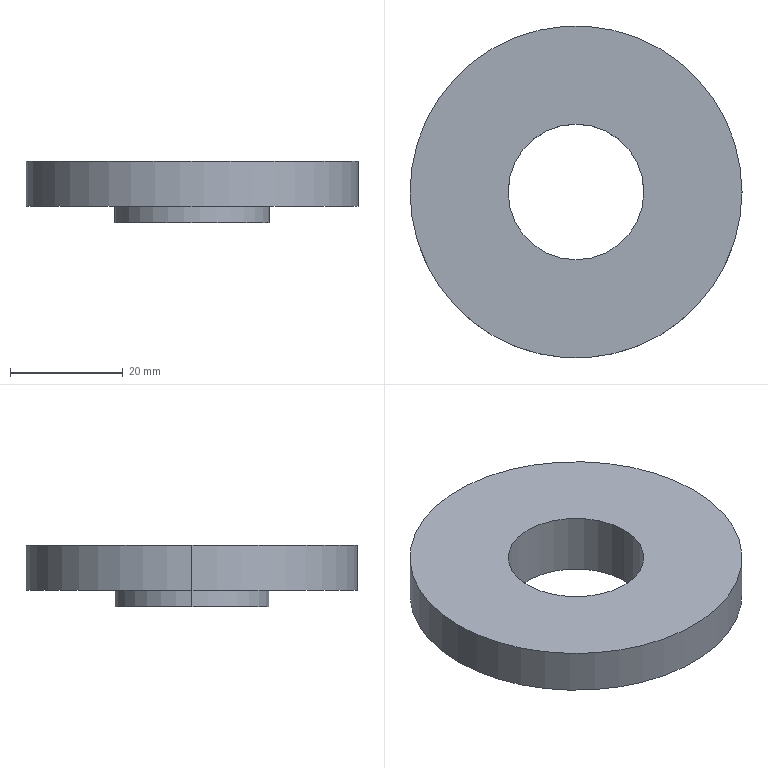Part | STEP file | LM-05-1133_default | 1 solid | 9 faces | box 59 x 59 x 11 mm | volume 18636 mm3 | cylinder 6 | plane 3 | commonest cylinder face diameters 24.1 x2 27.5 x2 59 x2
STEP:
#1=CARTESIAN_POINT('',(0.,0.,0.));
#2=DIRECTION('',(0.,0.,1.));
#3=DIRECTION('',(1.,0.,0.));
#4=AXIS2_PLACEMENT_3D('',#1,#2,#3);
#5=CARTESIAN_POINT('',(-13.75,0.,-2.));
#6=VERTEX_POINT('',#5);
#7=CARTESIAN_POINT('',(13.75,0.,-2.));
#8=VERTEX_POINT('',#7);
#9=CARTESIAN_POINT('',(0.,0.,-2.));
#10=DIRECTION('',(0.,0.,-1.));
#11=DIRECTION('',(-1.,0.,0.));
#12=AXIS2_PLACEMENT_3D('',#9,#10,#11);
#13=CIRCLE('',#12,13.75);
#14=CARTESIAN_POINT('',(0.,0.,6.));
#15=DIRECTION('',(0.,0.,-1.));
#16=DIRECTION('',(-1.,0.,0.));
#17=AXIS2_PLACEMENT_3D('',#14,#15,#16);
#18=CYLINDRICAL_SURFACE('',#17,13.75);
#19=CARTESIAN_POINT('',(0.,8.));
#20=DIRECTION('',(1.,0.));
#21=VECTOR('',#20,1.);
#22=LINE('',#19,#21);
#23=(GEOMETRIC_REPRESENTATION_CONTEXT(2)PARAMETRIC_REPRESENTATION_CONTEXT()REPRESENTATION_CONTEXT('',''));
#24=DEFINITIONAL_REPRESENTATION('',(#22),#23);
#25=PCURVE('',#18,#24);
#26=CARTESIAN_POINT('',(13.75,0.,-2.));
#27=DIRECTION('',(0.,0.,-1.));
#28=DIRECTION('',(-1.,0.,0.));
#29=AXIS2_PLACEMENT_3D('',#26,#27,#28);
#30=PLANE('',#29);
#31=CARTESIAN_POINT('',(13.75,0.));
#32=DIRECTION('',(1.,0.));
#33=AXIS2_PLACEMENT_2D('',#31,#32);
#34=CIRCLE('',#33,13.75);
#35=(GEOMETRIC_REPRESENTATION_CONTEXT(2)PARAMETRIC_REPRESENTATION_CONTEXT()REPRESENTATION_CONTEXT('',''));
#36=DEFINITIONAL_REPRESENTATION('',(#34),#35);
#37=PCURVE('',#30,#36);
#38=SURFACE_CURVE('',#13,(#25,#37),.PCURVE_S1.);
#39=EDGE_CURVE('',#6,#8,#38,.T.);
#40=ORIENTED_EDGE('',*,*,#39,.T.);
#41=CARTESIAN_POINT('',(13.75,0.,-5.));
#42=VERTEX_POINT('',#41);
#43=CARTESIAN_POINT('',(13.75,0.,6.));
#44=DIRECTION('',(0.,0.,-1.));
#45=VECTOR('',#44,1.);
#46=LINE('',#43,#45);
#47=CARTESIAN_POINT('',(3.142,0.));
#48=DIRECTION('',(0.,1.));
#49=VECTOR('',#48,1.);
#50=LINE('',#47,#49);
#51=(GEOMETRIC_REPRESENTATION_CONTEXT(2)PARAMETRIC_REPRESENTATION_CONTEXT()REPRESENTATION_CONTEXT('',''));
#52=DEFINITIONAL_REPRESENTATION('',(#50),#51);
#53=PCURVE('',#18,#52);
#54=CARTESIAN_POINT('',(0.,0.,6.));
#55=DIRECTION('',(0.,0.,-1.));
#56=DIRECTION('',(-1.,0.,0.));
#57=AXIS2_PLACEMENT_3D('',#54,#55,#56);
#58=CYLINDRICAL_SURFACE('',#57,13.75);
#59=CARTESIAN_POINT('',(3.142,0.));
#60=DIRECTION('',(0.,1.));
#61=VECTOR('',#60,1.);
#62=LINE('',#59,#61);
#63=(GEOMETRIC_REPRESENTATION_CONTEXT(2)PARAMETRIC_REPRESENTATION_CONTEXT()REPRESENTATION_CONTEXT('',''));
#64=DEFINITIONAL_REPRESENTATION('',(#62),#63);
#65=PCURVE('',#58,#64);
#66=SURFACE_CURVE('',#46,(#53,#65),.PCURVE_S1.);
#67=EDGE_CURVE('',#8,#42,#66,.T.);
#68=ORIENTED_EDGE('',*,*,#67,.T.);
#69=CARTESIAN_POINT('',(-13.75,0.,-5.));
#70=VERTEX_POINT('',#69);
#71=CARTESIAN_POINT('',(0.,0.,-5.));
#72=DIRECTION('',(0.,0.,-1.));
#73=DIRECTION('',(-1.,0.,0.));
#74=AXIS2_PLACEMENT_3D('',#71,#72,#73);
#75=CIRCLE('',#74,13.75);
#76=CARTESIAN_POINT('',(0.,11.));
#77=DIRECTION('',(1.,0.));
#78=VECTOR('',#77,1.);
#79=LINE('',#76,#78);
#80=(GEOMETRIC_REPRESENTATION_CONTEXT(2)PARAMETRIC_REPRESENTATION_CONTEXT()REPRESENTATION_CONTEXT('',''));
#81=DEFINITIONAL_REPRESENTATION('',(#79),#80);
#82=PCURVE('',#18,#81);
#83=CARTESIAN_POINT('',(12.05,0.,-5.));
#84=DIRECTION('',(0.,0.,-1.));
#85=DIRECTION('',(-1.,0.,0.));
#86=AXIS2_PLACEMENT_3D('',#83,#84,#85);
#87=PLANE('',#86);
#88=CARTESIAN_POINT('',(12.05,0.));
#89=DIRECTION('',(1.,0.));
#90=AXIS2_PLACEMENT_2D('',#88,#89);
#91=CIRCLE('',#90,13.75);
#92=(GEOMETRIC_REPRESENTATION_CONTEXT(2)PARAMETRIC_REPRESENTATION_CONTEXT()REPRESENTATION_CONTEXT('',''));
#93=DEFINITIONAL_REPRESENTATION('',(#91),#92);
#94=PCURVE('',#87,#93);
#95=SURFACE_CURVE('',#75,(#82,#94),.PCURVE_S1.);
#96=EDGE_CURVE('',#70,#42,#95,.T.);
#97=ORIENTED_EDGE('',*,*,#96,.F.);
#98=CARTESIAN_POINT('',(-13.75,0.,6.));
#99=DIRECTION('',(0.,0.,-1.));
#100=VECTOR('',#99,1.);
#101=LINE('',#98,#100);
#102=CARTESIAN_POINT('',(0.,0.));
#103=DIRECTION('',(0.,1.));
#104=VECTOR('',#103,1.);
#105=LINE('',#102,#104);
#106=(GEOMETRIC_REPRESENTATION_CONTEXT(2)PARAMETRIC_REPRESENTATION_CONTEXT()REPRESENTATION_CONTEXT('',''));
#107=DEFINITIONAL_REPRESENTATION('',(#105),#106);
#108=PCURVE('',#18,#107);
#109=CARTESIAN_POINT('',(6.283,0.));
#110=DIRECTION('',(0.,1.));
#111=VECTOR('',#110,1.);
#112=LINE('',#109,#111);
#113=(GEOMETRIC_REPRESENTATION_CONTEXT(2)PARAMETRIC_REPRESENTATION_CONTEXT()REPRESENTATION_CONTEXT('',''));
#114=DEFINITIONAL_REPRESENTATION('',(#112),#113);
#115=PCURVE('',#58,#114);
#116=SURFACE_CURVE('',#101,(#108,#115),.PCURVE_S1.);
#117=EDGE_CURVE('',#6,#70,#116,.T.);
#118=ORIENTED_EDGE('',*,*,#117,.F.);
#119=EDGE_LOOP('',(#40,#68,#97,#118));
#120=FACE_BOUND('',#119,.T.);
#121=ADVANCED_FACE('',(#120),#18,.T.);
#122=CARTESIAN_POINT('',(-12.05,0.,6.));
#123=VERTEX_POINT('',#122);
#124=CARTESIAN_POINT('',(-12.05,0.,-5.));
#125=VERTEX_POINT('',#124);
#126=CARTESIAN_POINT('',(-12.05,0.,6.));
#127=DIRECTION('',(0.,0.,-1.));
#128=VECTOR('',#127,1.);
#129=LINE('',#126,#128);
#130=CARTESIAN_POINT('',(0.,0.,6.));
#131=DIRECTION('',(0.,0.,-1.));
#132=DIRECTION('',(-1.,0.,0.));
#133=AXIS2_PLACEMENT_3D('',#130,#131,#132);
#134=CYLINDRICAL_SURFACE('',#133,12.05);
#135=CARTESIAN_POINT('',(6.283,0.));
#136=DIRECTION('',(0.,1.));
#137=VECTOR('',#136,1.);
#138=LINE('',#135,#137);
#139=(GEOMETRIC_REPRESENTATION_CONTEXT(2)PARAMETRIC_REPRESENTATION_CONTEXT()REPRESENTATION_CONTEXT('',''));
#140=DEFINITIONAL_REPRESENTATION('',(#138),#139);
#141=PCURVE('',#134,#140);
#142=CARTESIAN_POINT('',(0.,0.,6.));
#143=DIRECTION('',(0.,0.,-1.));
#144=DIRECTION('',(-1.,0.,0.));
#145=AXIS2_PLACEMENT_3D('',#142,#143,#144);
#146=CYLINDRICAL_SURFACE('',#145,12.05);
#147=CARTESIAN_POINT('',(0.,0.));
#148=DIRECTION('',(0.,1.));
#149=VECTOR('',#148,1.);
#150=LINE('',#147,#149);
#151=(GEOMETRIC_REPRESENTATION_CONTEXT(2)PARAMETRIC_REPRESENTATION_CONTEXT()REPRESENTATION_CONTEXT('',''));
#152=DEFINITIONAL_REPRESENTATION('',(#150),#151);
#153=PCURVE('',#146,#152);
#154=SURFACE_CURVE('',#129,(#141,#153),.PCURVE_S1.);
#155=EDGE_CURVE('',#123,#125,#154,.T.);
#156=ORIENTED_EDGE('',*,*,#155,.T.);
#157=CARTESIAN_POINT('',(12.05,0.,-5.));
#158=VERTEX_POINT('',#157);
#159=CARTESIAN_POINT('',(0.,0.,-5.));
#160=DIRECTION('',(0.,0.,-1.));
#161=DIRECTION('',(-1.,0.,0.));
#162=AXIS2_PLACEMENT_3D('',#159,#160,#161);
#163=CIRCLE('',#162,12.05);
#164=CARTESIAN_POINT('',(0.,11.));
#165=DIRECTION('',(1.,0.));
#166=VECTOR('',#165,1.);
#167=LINE('',#164,#166);
#168=(GEOMETRIC_REPRESENTATION_CONTEXT(2)PARAMETRIC_REPRESENTATION_CONTEXT()REPRESENTATION_CONTEXT('',''));
#169=DEFINITIONAL_REPRESENTATION('',(#167),#168);
#170=PCURVE('',#134,#169);
#171=CARTESIAN_POINT('',(12.05,0.));
#172=DIRECTION('',(1.,0.));
#173=AXIS2_PLACEMENT_2D('',#171,#172);
#174=CIRCLE('',#173,12.05);
#175=(GEOMETRIC_REPRESENTATION_CONTEXT(2)PARAMETRIC_REPRESENTATION_CONTEXT()REPRESENTATION_CONTEXT('',''));
#176=DEFINITIONAL_REPRESENTATION('',(#174),#175);
#177=PCURVE('',#87,#176);
#178=SURFACE_CURVE('',#163,(#170,#177),.PCURVE_S1.);
#179=EDGE_CURVE('',#158,#125,#178,.T.);
#180=ORIENTED_EDGE('',*,*,#179,.F.);
#181=CARTESIAN_POINT('',(12.05,0.,6.));
#182=VERTEX_POINT('',#181);
#183=CARTESIAN_POINT('',(12.05,0.,6.));
#184=DIRECTION('',(0.,0.,-1.));
#185=VECTOR('',#184,1.);
#186=LINE('',#183,#185);
#187=CARTESIAN_POINT('',(3.142,0.));
#188=DIRECTION('',(0.,1.));
#189=VECTOR('',#188,1.);
#190=LINE('',#187,#189);
#191=(GEOMETRIC_REPRESENTATION_CONTEXT(2)PARAMETRIC_REPRESENTATION_CONTEXT()REPRESENTATION_CONTEXT('',''));
#192=DEFINITIONAL_REPRESENTATION('',(#190),#191);
#193=PCURVE('',#134,#192);
#194=CARTESIAN_POINT('',(3.142,0.));
#195=DIRECTION('',(0.,1.));
#196=VECTOR('',#195,1.);
#197=LINE('',#194,#196);
#198=(GEOMETRIC_REPRESENTATION_CONTEXT(2)PARAMETRIC_REPRESENTATION_CONTEXT()REPRESENTATION_CONTEXT('',''));
#199=DEFINITIONAL_REPRESENTATION('',(#197),#198);
#200=PCURVE('',#146,#199);
#201=SURFACE_CURVE('',#186,(#193,#200),.PCURVE_S1.);
#202=EDGE_CURVE('',#182,#158,#201,.T.);
#203=ORIENTED_EDGE('',*,*,#202,.F.);
#204=CARTESIAN_POINT('',(0.,0.,6.));
#205=DIRECTION('',(0.,0.,-1.));
#206=DIRECTION('',(-1.,0.,0.));
#207=AXIS2_PLACEMENT_3D('',#204,#205,#206);
#208=CIRCLE('',#207,12.05);
#209=CARTESIAN_POINT('',(0.,0.));
#210=DIRECTION('',(1.,0.));
#211=VECTOR('',#210,1.);
#212=LINE('',#209,#211);
#213=(GEOMETRIC_REPRESENTATION_CONTEXT(2)PARAMETRIC_REPRESENTATION_CONTEXT()REPRESENTATION_CONTEXT('',''));
#214=DEFINITIONAL_REPRESENTATION('',(#212),#213);
#215=PCURVE('',#134,#214);
#216=CARTESIAN_POINT('',(29.5,0.,6.));
#217=DIRECTION('',(0.,0.,1.));
#218=DIRECTION('',(1.,0.,0.));
#219=AXIS2_PLACEMENT_3D('',#216,#217,#218);
#220=PLANE('',#219);
#221=CARTESIAN_POINT('',(-41.55,0.));
#222=CARTESIAN_POINT('',(-41.55,20.871));
#223=CARTESIAN_POINT('',(-23.475,10.436));
#224=CARTESIAN_POINT('',(-5.4,0.));
#225=CARTESIAN_POINT('',(-23.475,-10.436));
#226=CARTESIAN_POINT('',(-41.55,-20.871));
#227=CARTESIAN_POINT('',(-41.55,0.));
#228=(BOUNDED_CURVE()B_SPLINE_CURVE(2,(#221,#222,#223,#224,#225,#226,#227),.UNSPECIFIED.,.T.,.F.)B_SPLINE_CURVE_WITH_KNOTS((1,2,2,2,2,1),(-2.094,0.,2.094,4.189,6.283,8.378),.UNSPECIFIED.)CURVE()GEOMETRIC_REPRESENTATION_ITEM()RATIONAL_B_SPLINE_CURVE((1.,0.5,1.,0.5,1.,0.5,1.))REPRESENTATION_ITEM(''));
#229=(GEOMETRIC_REPRESENTATION_CONTEXT(2)PARAMETRIC_REPRESENTATION_CONTEXT()REPRESENTATION_CONTEXT('',''));
#230=DEFINITIONAL_REPRESENTATION('',(#228),#229);
#231=PCURVE('',#220,#230);
#232=SURFACE_CURVE('',#208,(#215,#231),.PCURVE_S1.);
#233=EDGE_CURVE('',#182,#123,#232,.T.);
#234=ORIENTED_EDGE('',*,*,#233,.T.);
#235=EDGE_LOOP('',(#156,#180,#203,#234));
#236=FACE_BOUND('',#235,.F.);
#237=ADVANCED_FACE('',(#236),#134,.F.);
#238=CARTESIAN_POINT('',(-29.5,0.,6.));
#239=VERTEX_POINT('',#238);
#240=CARTESIAN_POINT('',(29.5,0.,6.));
#241=VERTEX_POINT('',#240);
#242=CARTESIAN_POINT('',(0.,0.,6.));
#243=DIRECTION('',(0.,0.,-1.));
#244=DIRECTION('',(-1.,0.,0.));
#245=AXIS2_PLACEMENT_3D('',#242,#243,#244);
#246=CIRCLE('',#245,29.5);
#247=CARTESIAN_POINT('',(0.,0.,6.));
#248=DIRECTION('',(0.,0.,-1.));
#249=DIRECTION('',(-1.,0.,0.));
#250=AXIS2_PLACEMENT_3D('',#247,#248,#249);
#251=CYLINDRICAL_SURFACE('',#250,29.5);
#252=CARTESIAN_POINT('',(0.,0.));
#253=DIRECTION('',(1.,0.));
#254=VECTOR('',#253,1.);
#255=LINE('',#252,#254);
#256=(GEOMETRIC_REPRESENTATION_CONTEXT(2)PARAMETRIC_REPRESENTATION_CONTEXT()REPRESENTATION_CONTEXT('',''));
#257=DEFINITIONAL_REPRESENTATION('',(#255),#256);
#258=PCURVE('',#251,#257);
#259=CARTESIAN_POINT('',(-59.,0.));
#260=CARTESIAN_POINT('',(-59.,51.095));
#261=CARTESIAN_POINT('',(-14.75,25.548));
#262=CARTESIAN_POINT('',(29.5,0.));
#263=CARTESIAN_POINT('',(-14.75,-25.548));
#264=CARTESIAN_POINT('',(-59.,-51.095));
#265=CARTESIAN_POINT('',(-59.,0.));
#266=(BOUNDED_CURVE()B_SPLINE_CURVE(2,(#259,#260,#261,#262,#263,#264,#265),.UNSPECIFIED.,.T.,.F.)B_SPLINE_CURVE_WITH_KNOTS((1,2,2,2,2,1),(-2.094,0.,2.094,4.189,6.283,8.378),.UNSPECIFIED.)CURVE()GEOMETRIC_REPRESENTATION_ITEM()RATIONAL_B_SPLINE_CURVE((1.,0.5,1.,0.5,1.,0.5,1.))REPRESENTATION_ITEM(''));
#267=(GEOMETRIC_REPRESENTATION_CONTEXT(2)PARAMETRIC_REPRESENTATION_CONTEXT()REPRESENTATION_CONTEXT('',''));
#268=DEFINITIONAL_REPRESENTATION('',(#266),#267);
#269=PCURVE('',#220,#268);
#270=SURFACE_CURVE('',#246,(#258,#269),.PCURVE_S1.);
#271=EDGE_CURVE('',#239,#241,#270,.T.);
#272=ORIENTED_EDGE('',*,*,#271,.T.);
#273=CARTESIAN_POINT('',(29.5,0.,-2.));
#274=VERTEX_POINT('',#273);
#275=CARTESIAN_POINT('',(29.5,0.,6.));
#276=DIRECTION('',(0.,0.,-1.));
#277=VECTOR('',#276,1.);
#278=LINE('',#275,#277);
#279=CARTESIAN_POINT('',(3.142,0.));
#280=DIRECTION('',(0.,1.));
#281=VECTOR('',#280,1.);
#282=LINE('',#279,#281);
#283=(GEOMETRIC_REPRESENTATION_CONTEXT(2)PARAMETRIC_REPRESENTATION_CONTEXT()REPRESENTATION_CONTEXT('',''));
#284=DEFINITIONAL_REPRESENTATION('',(#282),#283);
#285=PCURVE('',#251,#284);
#286=CARTESIAN_POINT('',(0.,0.,6.));
#287=DIRECTION('',(0.,0.,-1.));
#288=DIRECTION('',(-1.,0.,0.));
#289=AXIS2_PLACEMENT_3D('',#286,#287,#288);
#290=CYLINDRICAL_SURFACE('',#289,29.5);
#291=CARTESIAN_POINT('',(3.142,0.));
#292=DIRECTION('',(0.,1.));
#293=VECTOR('',#292,1.);
#294=LINE('',#291,#293);
#295=(GEOMETRIC_REPRESENTATION_CONTEXT(2)PARAMETRIC_REPRESENTATION_CONTEXT()REPRESENTATION_CONTEXT('',''));
#296=DEFINITIONAL_REPRESENTATION('',(#294),#295);
#297=PCURVE('',#290,#296);
#298=SURFACE_CURVE('',#278,(#285,#297),.PCURVE_S1.);
#299=EDGE_CURVE('',#241,#274,#298,.T.);
#300=ORIENTED_EDGE('',*,*,#299,.T.);
#301=CARTESIAN_POINT('',(-29.5,0.,-2.));
#302=VERTEX_POINT('',#301);
#303=CARTESIAN_POINT('',(0.,0.,-2.));
#304=DIRECTION('',(0.,0.,-1.));
#305=DIRECTION('',(-1.,0.,0.));
#306=AXIS2_PLACEMENT_3D('',#303,#304,#305);
#307=CIRCLE('',#306,29.5);
#308=CARTESIAN_POINT('',(0.,8.));
#309=DIRECTION('',(1.,0.));
#310=VECTOR('',#309,1.);
#311=LINE('',#308,#310);
#312=(GEOMETRIC_REPRESENTATION_CONTEXT(2)PARAMETRIC_REPRESENTATION_CONTEXT()REPRESENTATION_CONTEXT('',''));
#313=DEFINITIONAL_REPRESENTATION('',(#311),#312);
#314=PCURVE('',#251,#313);
#315=CARTESIAN_POINT('',(13.75,0.));
#316=DIRECTION('',(1.,0.));
#317=AXIS2_PLACEMENT_2D('',#315,#316);
#318=CIRCLE('',#317,29.5);
#319=(GEOMETRIC_REPRESENTATION_CONTEXT(2)PARAMETRIC_REPRESENTATION_CONTEXT()REPRESENTATION_CONTEXT('',''));
#320=DEFINITIONAL_REPRESENTATION('',(#318),#319);
#321=PCURVE('',#30,#320);
#322=SURFACE_CURVE('',#307,(#314,#321),.PCURVE_S1.);
#323=EDGE_CURVE('',#302,#274,#322,.T.);
#324=ORIENTED_EDGE('',*,*,#323,.F.);
#325=CARTESIAN_POINT('',(-29.5,0.,6.));
#326=DIRECTION('',(0.,0.,-1.));
#327=VECTOR('',#326,1.);
#328=LINE('',#325,#327);
#329=CARTESIAN_POINT('',(0.,0.));
#330=DIRECTION('',(0.,1.));
#331=VECTOR('',#330,1.);
#332=LINE('',#329,#331);
#333=(GEOMETRIC_REPRESENTATION_CONTEXT(2)PARAMETRIC_REPRESENTATION_CONTEXT()REPRESENTATION_CONTEXT('',''));
#334=DEFINITIONAL_REPRESENTATION('',(#332),#333);
#335=PCURVE('',#251,#334);
#336=CARTESIAN_POINT('',(6.283,0.));
#337=DIRECTION('',(0.,1.));
#338=VECTOR('',#337,1.);
#339=LINE('',#336,#338);
#340=(GEOMETRIC_REPRESENTATION_CONTEXT(2)PARAMETRIC_REPRESENTATION_CONTEXT()REPRESENTATION_CONTEXT('',''));
#341=DEFINITIONAL_REPRESENTATION('',(#339),#340);
#342=PCURVE('',#290,#341);
#343=SURFACE_CURVE('',#328,(#335,#342),.PCURVE_S1.);
#344=EDGE_CURVE('',#239,#302,#343,.T.);
#345=ORIENTED_EDGE('',*,*,#344,.F.);
#346=EDGE_LOOP('',(#272,#300,#324,#345));
#347=FACE_BOUND('',#346,.T.);
#348=ADVANCED_FACE('',(#347),#251,.T.);
#349=ORIENTED_EDGE('',*,*,#299,.F.);
#350=CARTESIAN_POINT('',(0.,0.,6.));
#351=DIRECTION('',(0.,0.,-1.));
#352=DIRECTION('',(-1.,0.,0.));
#353=AXIS2_PLACEMENT_3D('',#350,#351,#352);
#354=CIRCLE('',#353,29.5);
#355=CARTESIAN_POINT('',(0.,0.));
#356=DIRECTION('',(1.,0.));
#357=VECTOR('',#356,1.);
#358=LINE('',#355,#357);
#359=(GEOMETRIC_REPRESENTATION_CONTEXT(2)PARAMETRIC_REPRESENTATION_CONTEXT()REPRESENTATION_CONTEXT('',''));
#360=DEFINITIONAL_REPRESENTATION('',(#358),#359);
#361=PCURVE('',#290,#360);
#362=CARTESIAN_POINT('',(-59.,0.));
#363=CARTESIAN_POINT('',(-59.,51.095));
#364=CARTESIAN_POINT('',(-14.75,25.548));
#365=CARTESIAN_POINT('',(29.5,0.));
#366=CARTESIAN_POINT('',(-14.75,-25.548));
#367=CARTESIAN_POINT('',(-59.,-51.095));
#368=CARTESIAN_POINT('',(-59.,0.));
#369=(BOUNDED_CURVE()B_SPLINE_CURVE(2,(#362,#363,#364,#365,#366,#367,#368),.UNSPECIFIED.,.T.,.F.)B_SPLINE_CURVE_WITH_KNOTS((1,2,2,2,2,1),(-2.094,0.,2.094,4.189,6.283,8.378),.UNSPECIFIED.)CURVE()GEOMETRIC_REPRESENTATION_ITEM()RATIONAL_B_SPLINE_CURVE((1.,0.5,1.,0.5,1.,0.5,1.))REPRESENTATION_ITEM(''));
#370=(GEOMETRIC_REPRESENTATION_CONTEXT(2)PARAMETRIC_REPRESENTATION_CONTEXT()REPRESENTATION_CONTEXT('',''));
#371=DEFINITIONAL_REPRESENTATION('',(#369),#370);
#372=PCURVE('',#220,#371);
#373=SURFACE_CURVE('',#354,(#361,#372),.PCURVE_S1.);
#374=EDGE_CURVE('',#241,#239,#373,.T.);
#375=ORIENTED_EDGE('',*,*,#374,.T.);
#376=ORIENTED_EDGE('',*,*,#344,.T.);
#377=CARTESIAN_POINT('',(0.,0.,-2.));
#378=DIRECTION('',(0.,0.,-1.));
#379=DIRECTION('',(-1.,0.,0.));
#380=AXIS2_PLACEMENT_3D('',#377,#378,#379);
#381=CIRCLE('',#380,29.5);
#382=CARTESIAN_POINT('',(0.,8.));
#383=DIRECTION('',(1.,0.));
#384=VECTOR('',#383,1.);
#385=LINE('',#382,#384);
#386=(GEOMETRIC_REPRESENTATION_CONTEXT(2)PARAMETRIC_REPRESENTATION_CONTEXT()REPRESENTATION_CONTEXT('',''));
#387=DEFINITIONAL_REPRESENTATION('',(#385),#386);
#388=PCURVE('',#290,#387);
#389=CARTESIAN_POINT('',(13.75,0.));
#390=DIRECTION('',(1.,0.));
#391=AXIS2_PLACEMENT_2D('',#389,#390);
#392=CIRCLE('',#391,29.5);
#393=(GEOMETRIC_REPRESENTATION_CONTEXT(2)PARAMETRIC_REPRESENTATION_CONTEXT()REPRESENTATION_CONTEXT('',''));
#394=DEFINITIONAL_REPRESENTATION('',(#392),#393);
#395=PCURVE('',#30,#394);
#396=SURFACE_CURVE('',#381,(#388,#395),.PCURVE_S1.);
#397=EDGE_CURVE('',#274,#302,#396,.T.);
#398=ORIENTED_EDGE('',*,*,#397,.F.);
#399=EDGE_LOOP('',(#349,#375,#376,#398));
#400=FACE_BOUND('',#399,.T.);
#401=ADVANCED_FACE('',(#400),#290,.T.);
#402=CARTESIAN_POINT('',(0.,0.,6.));
#403=DIRECTION('',(0.,0.,-1.));
#404=DIRECTION('',(-1.,0.,0.));
#405=AXIS2_PLACEMENT_3D('',#402,#403,#404);
#406=CIRCLE('',#405,12.05);
#407=CARTESIAN_POINT('',(-41.55,0.));
#408=CARTESIAN_POINT('',(-41.55,20.871));
#409=CARTESIAN_POINT('',(-23.475,10.436));
#410=CARTESIAN_POINT('',(-5.4,0.));
#411=CARTESIAN_POINT('',(-23.475,-10.436));
#412=CARTESIAN_POINT('',(-41.55,-20.871));
#413=CARTESIAN_POINT('',(-41.55,0.));
#414=(BOUNDED_CURVE()B_SPLINE_CURVE(2,(#407,#408,#409,#410,#411,#412,#413),.UNSPECIFIED.,.T.,.F.)B_SPLINE_CURVE_WITH_KNOTS((1,2,2,2,2,1),(-2.094,0.,2.094,4.189,6.283,8.378),.UNSPECIFIED.)CURVE()GEOMETRIC_REPRESENTATION_ITEM()RATIONAL_B_SPLINE_CURVE((1.,0.5,1.,0.5,1.,0.5,1.))REPRESENTATION_ITEM(''));
#415=(GEOMETRIC_REPRESENTATION_CONTEXT(2)PARAMETRIC_REPRESENTATION_CONTEXT()REPRESENTATION_CONTEXT('',''));
#416=DEFINITIONAL_REPRESENTATION('',(#414),#415);
#417=PCURVE('',#220,#416);
#418=CARTESIAN_POINT('',(0.,0.));
#419=DIRECTION('',(1.,0.));
#420=VECTOR('',#419,1.);
#421=LINE('',#418,#420);
#422=(GEOMETRIC_REPRESENTATION_CONTEXT(2)PARAMETRIC_REPRESENTATION_CONTEXT()REPRESENTATION_CONTEXT('',''));
#423=DEFINITIONAL_REPRESENTATION('',(#421),#422);
#424=PCURVE('',#146,#423);
#425=SURFACE_CURVE('',#406,(#417,#424),.PCURVE_S1.);
#426=EDGE_CURVE('',#123,#182,#425,.T.);
#427=ORIENTED_EDGE('',*,*,#426,.T.);
#428=ORIENTED_EDGE('',*,*,#233,.T.);
#429=EDGE_LOOP('',(#427,#428));
#430=FACE_BOUND('',#429,.T.);
#431=ORIENTED_EDGE('',*,*,#271,.F.);
#432=ORIENTED_EDGE('',*,*,#374,.F.);
#433=EDGE_LOOP('',(#431,#432));
#434=FACE_BOUND('',#433,.T.);
#435=ADVANCED_FACE('',(#430,#434),#220,.T.);
#436=CARTESIAN_POINT('',(0.,0.,-5.));
#437=DIRECTION('',(0.,0.,-1.));
#438=DIRECTION('',(-1.,0.,0.));
#439=AXIS2_PLACEMENT_3D('',#436,#437,#438);
#440=CIRCLE('',#439,12.05);
#441=CARTESIAN_POINT('',(0.,11.));
#442=DIRECTION('',(1.,0.));
#443=VECTOR('',#442,1.);
#444=LINE('',#441,#443);
#445=(GEOMETRIC_REPRESENTATION_CONTEXT(2)PARAMETRIC_REPRESENTATION_CONTEXT()REPRESENTATION_CONTEXT('',''));
#446=DEFINITIONAL_REPRESENTATION('',(#444),#445);
#447=PCURVE('',#146,#446);
#448=CARTESIAN_POINT('',(12.05,0.));
#449=DIRECTION('',(1.,0.));
#450=AXIS2_PLACEMENT_2D('',#448,#449);
#451=CIRCLE('',#450,12.05);
#452=(GEOMETRIC_REPRESENTATION_CONTEXT(2)PARAMETRIC_REPRESENTATION_CONTEXT()REPRESENTATION_CONTEXT('',''));
#453=DEFINITIONAL_REPRESENTATION('',(#451),#452);
#454=PCURVE('',#87,#453);
#455=SURFACE_CURVE('',#440,(#447,#454),.PCURVE_S1.);
#456=EDGE_CURVE('',#125,#158,#455,.T.);
#457=ORIENTED_EDGE('',*,*,#456,.F.);
#458=ORIENTED_EDGE('',*,*,#155,.F.);
#459=ORIENTED_EDGE('',*,*,#426,.T.);
#460=ORIENTED_EDGE('',*,*,#202,.T.);
#461=EDGE_LOOP('',(#457,#458,#459,#460));
#462=FACE_BOUND('',#461,.F.);
#463=ADVANCED_FACE('',(#462),#146,.F.);
#464=ORIENTED_EDGE('',*,*,#96,.T.);
#465=CARTESIAN_POINT('',(0.,0.,-5.));
#466=DIRECTION('',(0.,0.,-1.));
#467=DIRECTION('',(-1.,0.,0.));
#468=AXIS2_PLACEMENT_3D('',#465,#466,#467);
#469=CIRCLE('',#468,13.75);
#470=CARTESIAN_POINT('',(12.05,0.));
#471=DIRECTION('',(1.,0.));
#472=AXIS2_PLACEMENT_2D('',#470,#471);
#473=CIRCLE('',#472,13.75);
#474=(GEOMETRIC_REPRESENTATION_CONTEXT(2)PARAMETRIC_REPRESENTATION_CONTEXT()REPRESENTATION_CONTEXT('',''));
#475=DEFINITIONAL_REPRESENTATION('',(#473),#474);
#476=PCURVE('',#87,#475);
#477=CARTESIAN_POINT('',(0.,11.));
#478=DIRECTION('',(1.,0.));
#479=VECTOR('',#478,1.);
#480=LINE('',#477,#479);
#481=(GEOMETRIC_REPRESENTATION_CONTEXT(2)PARAMETRIC_REPRESENTATION_CONTEXT()REPRESENTATION_CONTEXT('',''));
#482=DEFINITIONAL_REPRESENTATION('',(#480),#481);
#483=PCURVE('',#58,#482);
#484=SURFACE_CURVE('',#469,(#476,#483),.PCURVE_S1.);
#485=EDGE_CURVE('',#42,#70,#484,.T.);
#486=ORIENTED_EDGE('',*,*,#485,.T.);
#487=EDGE_LOOP('',(#464,#486));
#488=FACE_BOUND('',#487,.T.);
#489=ORIENTED_EDGE('',*,*,#456,.F.);
#490=ORIENTED_EDGE('',*,*,#179,.F.);
#491=EDGE_LOOP('',(#489,#490));
#492=FACE_BOUND('',#491,.T.);
#493=ADVANCED_FACE('',(#488,#492),#87,.T.);
#494=ORIENTED_EDGE('',*,*,#67,.F.);
#495=CARTESIAN_POINT('',(0.,0.,-2.));
#496=DIRECTION('',(0.,0.,-1.));
#497=DIRECTION('',(-1.,0.,0.));
#498=AXIS2_PLACEMENT_3D('',#495,#496,#497);
#499=CIRCLE('',#498,13.75);
#500=CARTESIAN_POINT('',(0.,8.));
#501=DIRECTION('',(1.,0.));
#502=VECTOR('',#501,1.);
#503=LINE('',#500,#502);
#504=(GEOMETRIC_REPRESENTATION_CONTEXT(2)PARAMETRIC_REPRESENTATION_CONTEXT()REPRESENTATION_CONTEXT('',''));
#505=DEFINITIONAL_REPRESENTATION('',(#503),#504);
#506=PCURVE('',#58,#505);
#507=CARTESIAN_POINT('',(13.75,0.));
#508=DIRECTION('',(1.,0.));
#509=AXIS2_PLACEMENT_2D('',#507,#508);
#510=CIRCLE('',#509,13.75);
#511=(GEOMETRIC_REPRESENTATION_CONTEXT(2)PARAMETRIC_REPRESENTATION_CONTEXT()REPRESENTATION_CONTEXT('',''));
#512=DEFINITIONAL_REPRESENTATION('',(#510),#511);
#513=PCURVE('',#30,#512);
#514=SURFACE_CURVE('',#499,(#506,#513),.PCURVE_S1.);
#515=EDGE_CURVE('',#8,#6,#514,.T.);
#516=ORIENTED_EDGE('',*,*,#515,.T.);
#517=ORIENTED_EDGE('',*,*,#117,.T.);
#518=ORIENTED_EDGE('',*,*,#485,.F.);
#519=EDGE_LOOP('',(#494,#516,#517,#518));
#520=FACE_BOUND('',#519,.T.);
#521=ADVANCED_FACE('',(#520),#58,.T.);
#522=ORIENTED_EDGE('',*,*,#323,.T.);
#523=ORIENTED_EDGE('',*,*,#397,.T.);
#524=EDGE_LOOP('',(#522,#523));
#525=FACE_BOUND('',#524,.T.);
#526=ORIENTED_EDGE('',*,*,#39,.F.);
#527=ORIENTED_EDGE('',*,*,#515,.F.);
#528=EDGE_LOOP('',(#526,#527));
#529=FACE_BOUND('',#528,.T.);
#530=ADVANCED_FACE('',(#525,#529),#30,.T.);
#531=CLOSED_SHELL('',(#121,#237,#348,#401,#435,#463,#493,#521,#530));
#532=MANIFOLD_SOLID_BREP('',#531);
#533=(LENGTH_UNIT()NAMED_UNIT(*)SI_UNIT(.MILLI.,.METRE.));
#534=UNCERTAINTY_MEASURE_WITH_UNIT(LENGTH_MEASURE(0.0000001),#533,'','');
#535=(NAMED_UNIT(*)PLANE_ANGLE_UNIT()SI_UNIT($,.RADIAN.));
#536=(NAMED_UNIT(*)SI_UNIT($,.STERADIAN.)SOLID_ANGLE_UNIT());
#537=(GEOMETRIC_REPRESENTATION_CONTEXT(3)GLOBAL_UNCERTAINTY_ASSIGNED_CONTEXT((#534))GLOBAL_UNIT_ASSIGNED_CONTEXT((#533,#535,#536))REPRESENTATION_CONTEXT('',''));
#538=ADVANCED_BREP_SHAPE_REPRESENTATION('',(#4,#532),#537);